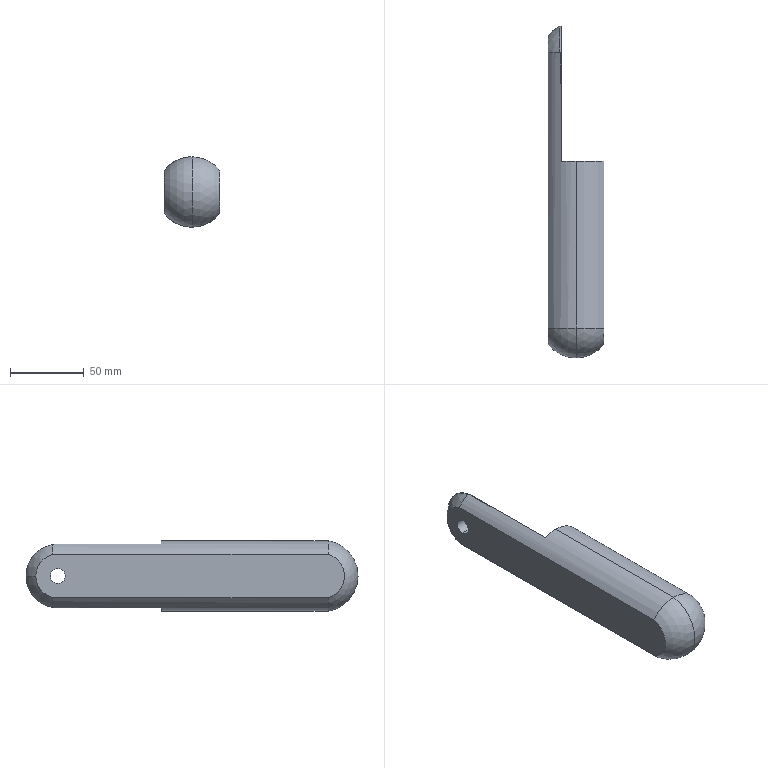Part | SolidWorks | features ICE 12, Fillet 4, RevCut 1, Revolution 1, Scale 1 | 1 solid | 18 faces | box 37.836 x 225.102 x 47.771 mm | volume 229671 mm3 | cylinder 7 | sphere 4 | plane 4 | spline 2 | torus 1 | commonest cylinder face diameters 47.771 x3 1.9 x2 10.1 x2
STEP:
#1=CARTESIAN_POINT('',(18.918,-183.171,14.582));
#2=VERTEX_POINT('',#1);
#3=CARTESIAN_POINT('',(0.,-183.171,23.885));
#4=VERTEX_POINT('',#3);
#5=CARTESIAN_POINT('',(0.,-183.171,0.));
#6=DIRECTION('',(0.,-1.,0.));
#7=DIRECTION('',(0.,0.,-1.));
#8=AXIS2_PLACEMENT_3D('',#5,#6,#7);
#9=CIRCLE('',#8,23.885);
#10=EDGE_CURVE('',#2,#4,#9,.T.);
#11=ORIENTED_EDGE('',*,*,#10,.T.);
#12=CARTESIAN_POINT('',(0.,-203.461,0.));
#13=VERTEX_POINT('',#12);
#14=CARTESIAN_POINT('',(0.,-179.257,0.));
#15=DIRECTION('',(1.,0.,0.));
#16=DIRECTION('',(0.,0.,-1.));
#17=AXIS2_PLACEMENT_3D('',#14,#15,#16);
#18=CIRCLE('',#17,24.204);
#19=EDGE_CURVE('',#4,#13,#18,.T.);
#20=ORIENTED_EDGE('',*,*,#19,.T.);
#21=CARTESIAN_POINT('',(0.,-183.171,-23.885));
#22=VERTEX_POINT('',#21);
#23=CARTESIAN_POINT('',(0.,-179.257,0.));
#24=DIRECTION('',(-1.,0.,0.));
#25=DIRECTION('',(0.,0.,1.));
#26=AXIS2_PLACEMENT_3D('',#23,#24,#25);
#27=CIRCLE('',#26,24.204);
#28=EDGE_CURVE('',#22,#13,#27,.T.);
#29=ORIENTED_EDGE('',*,*,#28,.F.);
#30=CARTESIAN_POINT('',(18.918,-183.171,-14.582));
#31=VERTEX_POINT('',#30);
#32=CARTESIAN_POINT('',(0.,-183.171,0.));
#33=DIRECTION('',(0.,-1.,0.));
#34=DIRECTION('',(0.,0.,-1.));
#35=AXIS2_PLACEMENT_3D('',#32,#33,#34);
#36=CIRCLE('',#35,23.885);
#37=EDGE_CURVE('',#22,#31,#36,.T.);
#38=ORIENTED_EDGE('',*,*,#37,.T.);
#39=CARTESIAN_POINT('',(18.918,-179.257,0.));
#40=DIRECTION('',(1.,0.,0.));
#41=DIRECTION('',(0.,0.,1.));
#42=AXIS2_PLACEMENT_3D('',#39,#40,#41);
#43=CIRCLE('',#42,15.098);
#44=EDGE_CURVE('',#2,#31,#43,.T.);
#45=ORIENTED_EDGE('',*,*,#44,.F.);
#46=EDGE_LOOP('',(#11,#20,#29,#38,#45));
#47=FACE_OUTER_BOUND('',#46,.T.);
#48=CARTESIAN_POINT('',(0.,-179.257,0.));
#49=DIRECTION('',(1.,0.,0.));
#50=DIRECTION('',(0.,0.,-1.));
#51=AXIS2_PLACEMENT_3D('',#48,#49,#50);
#52=SPHERICAL_SURFACE('',#51,24.204);
#53=ADVANCED_FACE('',(#47),#52,.T.);
#54=CARTESIAN_POINT('',(-10.,0.,5.05));
#55=VERTEX_POINT('',#54);
#56=CARTESIAN_POINT('',(-10.,0.,-5.05));
#57=VERTEX_POINT('',#56);
#58=CARTESIAN_POINT('',(-10.,0.,0.));
#59=DIRECTION('',(1.,0.,0.));
#60=DIRECTION('',(0.,0.,1.));
#61=AXIS2_PLACEMENT_3D('',#58,#59,#60);
#62=CIRCLE('',#61,5.05);
#63=EDGE_CURVE('',#55,#57,#62,.T.);
#64=ORIENTED_EDGE('',*,*,#63,.T.);
#65=CARTESIAN_POINT('',(-18.918,0.,-5.05));
#66=VERTEX_POINT('',#65);
#67=CARTESIAN_POINT('',(21.42,0.,-5.05));
#68=DIRECTION('',(-1.,0.,0.));
#69=VECTOR('',#68,1000.);
#70=LINE('',#67,#69);
#71=EDGE_CURVE('',#57,#66,#70,.T.);
#72=ORIENTED_EDGE('',*,*,#71,.T.);
#73=CARTESIAN_POINT('',(-18.918,0.,5.05));
#74=VERTEX_POINT('',#73);
#75=CARTESIAN_POINT('',(-18.918,0.,0.));
#76=DIRECTION('',(-1.,0.,0.));
#77=DIRECTION('',(0.,0.,-1.));
#78=AXIS2_PLACEMENT_3D('',#75,#76,#77);
#79=CIRCLE('',#78,5.05);
#80=EDGE_CURVE('',#66,#74,#79,.T.);
#81=ORIENTED_EDGE('',*,*,#80,.T.);
#82=CARTESIAN_POINT('',(21.42,0.,5.05));
#83=DIRECTION('',(-1.,0.,0.));
#84=VECTOR('',#83,1000.);
#85=LINE('',#82,#84);
#86=EDGE_CURVE('',#55,#74,#85,.T.);
#87=ORIENTED_EDGE('',*,*,#86,.F.);
#88=EDGE_LOOP('',(#64,#72,#81,#87));
#89=FACE_OUTER_BOUND('',#88,.T.);
#90=CARTESIAN_POINT('',(21.42,0.,0.));
#91=DIRECTION('',(-1.,0.,0.));
#92=DIRECTION('',(0.,0.,1.));
#93=AXIS2_PLACEMENT_3D('',#90,#91,#92);
#94=CYLINDRICAL_SURFACE('',#93,5.05);
#95=ADVANCED_FACE('',(#89),#94,.F.);
#96=CARTESIAN_POINT('',(-18.918,3.427,-14.582));
#97=VERTEX_POINT('',#96);
#98=CARTESIAN_POINT('',(-18.918,14.979,0.));
#99=VERTEX_POINT('',#98);
#100=CARTESIAN_POINT('',(-18.918,0.,0.));
#101=DIRECTION('',(1.,0.,0.));
#102=DIRECTION('',(0.,0.,-1.));
#103=AXIS2_PLACEMENT_3D('',#100,#101,#102);
#104=CIRCLE('',#103,14.979);
#105=EDGE_CURVE('',#97,#99,#104,.T.);
#106=ORIENTED_EDGE('',*,*,#105,.T.);
#107=CARTESIAN_POINT('',(-10.878,21.539,0.));
#108=VERTEX_POINT('',#107);
#109=CARTESIAN_POINT('',(0.,0.,0.));
#110=DIRECTION('',(0.,0.,-1.));
#111=DIRECTION('',(-1.,0.,0.));
#112=AXIS2_PLACEMENT_3D('',#109,#110,#111);
#113=CIRCLE('',#112,24.13);
#114=EDGE_CURVE('',#99,#108,#113,.T.);
#115=ORIENTED_EDGE('',*,*,#114,.T.);
#116=CARTESIAN_POINT('',(-10.878,3.427,-21.264));
#117=VERTEX_POINT('',#116);
#118=CARTESIAN_POINT('',(-10.878,0.,0.));
#119=DIRECTION('',(-1.,0.,0.));
#120=DIRECTION('',(0.,1.,0.));
#121=AXIS2_PLACEMENT_3D('',#118,#119,#120);
#122=CIRCLE('',#121,21.539);
#123=EDGE_CURVE('',#108,#117,#122,.T.);
#124=ORIENTED_EDGE('',*,*,#123,.T.);
#125=CARTESIAN_POINT('',(0.,3.427,0.));
#126=DIRECTION('',(0.,1.,0.));
#127=DIRECTION('',(0.,0.,-1.));
#128=AXIS2_PLACEMENT_3D('',#125,#126,#127);
#129=CIRCLE('',#128,23.885);
#130=EDGE_CURVE('',#117,#97,#129,.T.);
#131=ORIENTED_EDGE('',*,*,#130,.T.);
#132=EDGE_LOOP('',(#106,#115,#124,#131));
#133=FACE_OUTER_BOUND('',#132,.T.);
#134=CARTESIAN_POINT('',(0.,0.,0.));
#135=DIRECTION('',(0.,0.,-1.));
#136=DIRECTION('',(1.,0.,0.));
#137=AXIS2_PLACEMENT_3D('',#134,#135,#136);
#138=SPHERICAL_SURFACE('',#137,24.13);
#139=ADVANCED_FACE('',(#133),#138,.T.);
#140=CARTESIAN_POINT('',(-18.918,-183.171,14.582));
#141=VERTEX_POINT('',#140);
#142=CARTESIAN_POINT('',(0.,-183.171,0.));
#143=DIRECTION('',(0.,-1.,0.));
#144=DIRECTION('',(0.,0.,-1.));
#145=AXIS2_PLACEMENT_3D('',#142,#143,#144);
#146=CIRCLE('',#145,23.885);
#147=EDGE_CURVE('',#4,#141,#146,.T.);
#148=ORIENTED_EDGE('',*,*,#147,.F.);
#149=CARTESIAN_POINT('',(0.,-70.,23.885));
#150=VERTEX_POINT('',#149);
#151=CARTESIAN_POINT('',(0.,-127.87,23.885));
#152=DIRECTION('',(0.,1.,0.));
#153=VECTOR('',#152,1000.);
#154=LINE('',#151,#153);
#155=EDGE_CURVE('',#4,#150,#154,.T.);
#156=ORIENTED_EDGE('',*,*,#155,.T.);
#157=CARTESIAN_POINT('',(-10.,-70.,21.691));
#158=VERTEX_POINT('',#157);
#159=CARTESIAN_POINT('',(0.,-70.,0.));
#160=DIRECTION('',(0.,1.,0.));
#161=DIRECTION('',(0.,0.,-1.));
#162=AXIS2_PLACEMENT_3D('',#159,#160,#161);
#163=CIRCLE('',#162,23.885);
#164=EDGE_CURVE('',#158,#150,#163,.T.);
#165=ORIENTED_EDGE('',*,*,#164,.F.);
#166=CARTESIAN_POINT('',(-10.,-18.195,21.691));
#167=VERTEX_POINT('',#166);
#168=CARTESIAN_POINT('',(-10.,-127.87,21.691));
#169=DIRECTION('',(0.,-1.,0.));
#170=VECTOR('',#169,1000.);
#171=LINE('',#168,#170);
#172=EDGE_CURVE('',#167,#158,#171,.T.);
#173=ORIENTED_EDGE('',*,*,#172,.F.);
#174=CARTESIAN_POINT('',(-10.187,-17.296,21.604));
#175=VERTEX_POINT('',#174);
#176=CARTESIAN_POINT('',(-10.187,-17.296,21.604));
#177=CARTESIAN_POINT('',(-10.187,-17.452,21.604));
#178=CARTESIAN_POINT('',(-10.175,-17.607,21.61));
#179=CARTESIAN_POINT('',(-10.118,-17.909,21.636));
#180=CARTESIAN_POINT('',(-10.072,-18.06,21.658));
#181=CARTESIAN_POINT('',(-10.,-18.195,21.691));
#182=B_SPLINE_CURVE_WITH_KNOTS('',3,(#176,#177,#178,#179,#180,#181),.UNSPECIFIED.,.F.,.F.,(4,2,4),(0.,0.0004629,0.0009257),.UNSPECIFIED.);
#183=EDGE_CURVE('',#175,#167,#182,.T.);
#184=ORIENTED_EDGE('',*,*,#183,.F.);
#185=CARTESIAN_POINT('',(-10.187,0.,21.604));
#186=VERTEX_POINT('',#185);
#187=CARTESIAN_POINT('',(-10.187,-53.115,21.604));
#188=DIRECTION('',(0.,-1.,0.));
#189=VECTOR('',#188,1000.);
#190=LINE('',#187,#189);
#191=EDGE_CURVE('',#186,#175,#190,.T.);
#192=ORIENTED_EDGE('',*,*,#191,.F.);
#193=CARTESIAN_POINT('',(-10.878,3.427,21.264));
#194=VERTEX_POINT('',#193);
#195=CARTESIAN_POINT('',(-10.878,3.427,21.264));
#196=CARTESIAN_POINT('',(-10.844,3.427,21.282));
#197=CARTESIAN_POINT('',(-10.811,3.411,21.299));
#198=CARTESIAN_POINT('',(-10.755,3.366,21.327));
#199=CARTESIAN_POINT('',(-10.731,3.339,21.339));
#200=CARTESIAN_POINT('',(-10.667,3.249,21.371));
#201=CARTESIAN_POINT('',(-10.633,3.182,21.388));
#202=CARTESIAN_POINT('',(-10.543,2.979,21.433));
#203=CARTESIAN_POINT('',(-10.498,2.834,21.455));
#204=CARTESIAN_POINT('',(-10.384,2.398,21.51));
#205=CARTESIAN_POINT('',(-10.334,2.102,21.534));
#206=CARTESIAN_POINT('',(-10.218,1.21,21.59));
#207=CARTESIAN_POINT('',(-10.187,0.6043,21.604));
#208=CARTESIAN_POINT('',(-10.187,0.,21.604));
#209=B_SPLINE_CURVE_WITH_KNOTS('',3,(#195,#196,#197,#198,#199,#200,#201,#202,#203,#204,#205,#206,#207,#208),.UNSPECIFIED.,.F.,.F.,(4,2,2,2,2,2,4),(0.000000221,0.0001151,0.00023,0.0004598,0.0009194,0.001839,0.003677),.UNSPECIFIED.);
#210=EDGE_CURVE('',#194,#186,#209,.T.);
#211=ORIENTED_EDGE('',*,*,#210,.F.);
#212=CARTESIAN_POINT('',(-18.918,3.427,14.582));
#213=VERTEX_POINT('',#212);
#214=CARTESIAN_POINT('',(0.,3.427,0.));
#215=DIRECTION('',(0.,1.,0.));
#216=DIRECTION('',(0.,0.,-1.));
#217=AXIS2_PLACEMENT_3D('',#214,#215,#216);
#218=CIRCLE('',#217,23.885);
#219=EDGE_CURVE('',#213,#194,#218,.T.);
#220=ORIENTED_EDGE('',*,*,#219,.F.);
#221=CARTESIAN_POINT('',(-18.918,-127.87,14.582));
#222=DIRECTION('',(0.,1.,0.));
#223=VECTOR('',#222,1000.);
#224=LINE('',#221,#223);
#225=EDGE_CURVE('',#141,#213,#224,.T.);
#226=ORIENTED_EDGE('',*,*,#225,.F.);
#227=EDGE_LOOP('',(#148,#156,#165,#173,#184,#192,#211,#220,#226));
#228=FACE_OUTER_BOUND('',#227,.T.);
#229=CARTESIAN_POINT('',(0.,-127.87,0.));
#230=DIRECTION('',(0.,1.,0.));
#231=DIRECTION('',(0.,0.,1.));
#232=AXIS2_PLACEMENT_3D('',#229,#230,#231);
#233=CYLINDRICAL_SURFACE('',#232,23.885);
#234=ADVANCED_FACE('',(#228),#233,.T.);
#235=CARTESIAN_POINT('',(-18.918,-183.171,-14.582));
#236=VERTEX_POINT('',#235);
#237=CARTESIAN_POINT('',(-18.918,-127.87,-14.582));
#238=DIRECTION('',(0.,-1.,0.));
#239=VECTOR('',#238,1000.);
#240=LINE('',#237,#239);
#241=EDGE_CURVE('',#97,#236,#240,.T.);
#242=ORIENTED_EDGE('',*,*,#241,.F.);
#243=ORIENTED_EDGE('',*,*,#130,.F.);
#244=CARTESIAN_POINT('',(-10.187,0.,-21.604));
#245=VERTEX_POINT('',#244);
#246=CARTESIAN_POINT('',(-10.187,0.,-21.604));
#247=CARTESIAN_POINT('',(-10.187,0.6048,-21.604));
#248=CARTESIAN_POINT('',(-10.217,1.207,-21.59));
#249=CARTESIAN_POINT('',(-10.334,2.105,-21.534));
#250=CARTESIAN_POINT('',(-10.385,2.404,-21.51));
#251=CARTESIAN_POINT('',(-10.5,2.839,-21.454));
#252=CARTESIAN_POINT('',(-10.545,2.983,-21.432));
#253=CARTESIAN_POINT('',(-10.635,3.186,-21.387));
#254=CARTESIAN_POINT('',(-10.669,3.252,-21.37));
#255=CARTESIAN_POINT('',(-10.733,3.34,-21.338));
#256=CARTESIAN_POINT('',(-10.756,3.368,-21.326));
#257=CARTESIAN_POINT('',(-10.812,3.411,-21.298));
#258=CARTESIAN_POINT('',(-10.844,3.427,-21.282));
#259=CARTESIAN_POINT('',(-10.878,3.427,-21.264));
#260=B_SPLINE_CURVE_WITH_KNOTS('',3,(#246,#247,#248,#249,#250,#251,#252,#253,#254,#255,#256,#257,#258,#259),.UNSPECIFIED.,.F.,.F.,(4,2,2,2,2,2,4),(0.0000002,0.00181,0.002715,0.003167,0.003394,0.003507,0.00362),.UNSPECIFIED.);
#261=EDGE_CURVE('',#245,#117,#260,.T.);
#262=ORIENTED_EDGE('',*,*,#261,.F.);
#263=CARTESIAN_POINT('',(-10.187,-58.677,-21.604));
#264=VERTEX_POINT('',#263);
#265=CARTESIAN_POINT('',(-10.187,-53.115,-21.604));
#266=DIRECTION('',(0.,1.,0.));
#267=VECTOR('',#266,1000.);
#268=LINE('',#265,#267);
#269=EDGE_CURVE('',#264,#245,#268,.T.);
#270=ORIENTED_EDGE('',*,*,#269,.F.);
#271=CARTESIAN_POINT('',(-10.,-59.803,-21.691));
#272=VERTEX_POINT('',#271);
#273=CARTESIAN_POINT('',(-10.,-59.803,-21.691));
#274=CARTESIAN_POINT('',(-10.058,-59.623,-21.664));
#275=CARTESIAN_POINT('',(-10.105,-59.436,-21.643));
#276=CARTESIAN_POINT('',(-10.169,-59.061,-21.613));
#277=CARTESIAN_POINT('',(-10.187,-58.871,-21.604));
#278=CARTESIAN_POINT('',(-10.187,-58.677,-21.604));
#279=B_SPLINE_CURVE_WITH_KNOTS('',3,(#273,#274,#275,#276,#277,#278),.UNSPECIFIED.,.F.,.F.,(4,2,4),(0.00244,0.003016,0.003592),.UNSPECIFIED.);
#280=EDGE_CURVE('',#272,#264,#279,.T.);
#281=ORIENTED_EDGE('',*,*,#280,.F.);
#282=CARTESIAN_POINT('',(-10.,-70.,-21.691));
#283=VERTEX_POINT('',#282);
#284=CARTESIAN_POINT('',(-10.,-127.87,-21.691));
#285=DIRECTION('',(0.,1.,0.));
#286=VECTOR('',#285,1000.);
#287=LINE('',#284,#286);
#288=EDGE_CURVE('',#283,#272,#287,.T.);
#289=ORIENTED_EDGE('',*,*,#288,.F.);
#290=CARTESIAN_POINT('',(18.918,-70.,-14.582));
#291=VERTEX_POINT('',#290);
#292=CARTESIAN_POINT('',(0.,-70.,0.));
#293=DIRECTION('',(0.,1.,0.));
#294=DIRECTION('',(0.,0.,-1.));
#295=AXIS2_PLACEMENT_3D('',#292,#293,#294);
#296=CIRCLE('',#295,23.885);
#297=EDGE_CURVE('',#291,#283,#296,.T.);
#298=ORIENTED_EDGE('',*,*,#297,.F.);
#299=CARTESIAN_POINT('',(18.918,-127.87,-14.582));
#300=DIRECTION('',(0.,1.,0.));
#301=VECTOR('',#300,1000.);
#302=LINE('',#299,#301);
#303=EDGE_CURVE('',#31,#291,#302,.T.);
#304=ORIENTED_EDGE('',*,*,#303,.F.);
#305=ORIENTED_EDGE('',*,*,#37,.F.);
#306=CARTESIAN_POINT('',(0.,-183.171,0.));
#307=DIRECTION('',(0.,-1.,0.));
#308=DIRECTION('',(0.,0.,-1.));
#309=AXIS2_PLACEMENT_3D('',#306,#307,#308);
#310=CIRCLE('',#309,23.885);
#311=EDGE_CURVE('',#236,#22,#310,.T.);
#312=ORIENTED_EDGE('',*,*,#311,.F.);
#313=EDGE_LOOP('',(#242,#243,#262,#270,#281,#289,#298,#304,#305,#312));
#314=FACE_OUTER_BOUND('',#313,.T.);
#315=CARTESIAN_POINT('',(0.,-127.87,0.));
#316=DIRECTION('',(0.,1.,0.));
#317=DIRECTION('',(0.,0.,1.));
#318=AXIS2_PLACEMENT_3D('',#315,#316,#317);
#319=CYLINDRICAL_SURFACE('',#318,23.885);
#320=ADVANCED_FACE('',(#314),#319,.T.);
#321=ORIENTED_EDGE('',*,*,#155,.F.);
#322=ORIENTED_EDGE('',*,*,#10,.F.);
#323=CARTESIAN_POINT('',(18.918,-70.,14.582));
#324=VERTEX_POINT('',#323);
#325=CARTESIAN_POINT('',(18.918,-127.87,14.582));
#326=DIRECTION('',(0.,-1.,0.));
#327=VECTOR('',#326,1000.);
#328=LINE('',#325,#327);
#329=EDGE_CURVE('',#324,#2,#328,.T.);
#330=ORIENTED_EDGE('',*,*,#329,.F.);
#331=CARTESIAN_POINT('',(0.,-70.,0.));
#332=DIRECTION('',(0.,1.,0.));
#333=DIRECTION('',(0.,0.,-1.));
#334=AXIS2_PLACEMENT_3D('',#331,#332,#333);
#335=CIRCLE('',#334,23.885);
#336=EDGE_CURVE('',#150,#324,#335,.T.);
#337=ORIENTED_EDGE('',*,*,#336,.F.);
#338=EDGE_LOOP('',(#321,#322,#330,#337));
#339=FACE_OUTER_BOUND('',#338,.T.);
#340=CARTESIAN_POINT('',(0.,-127.87,0.));
#341=DIRECTION('',(0.,1.,0.));
#342=DIRECTION('',(0.,0.,1.));
#343=AXIS2_PLACEMENT_3D('',#340,#341,#342);
#344=CYLINDRICAL_SURFACE('',#343,23.885);
#345=ADVANCED_FACE('',(#339),#344,.T.);
#346=ORIENTED_EDGE('',*,*,#114,.F.);
#347=CARTESIAN_POINT('',(-18.918,0.,0.));
#348=DIRECTION('',(1.,0.,0.));
#349=DIRECTION('',(0.,0.,-1.));
#350=AXIS2_PLACEMENT_3D('',#347,#348,#349);
#351=CIRCLE('',#350,14.979);
#352=EDGE_CURVE('',#99,#213,#351,.T.);
#353=ORIENTED_EDGE('',*,*,#352,.T.);
#354=ORIENTED_EDGE('',*,*,#219,.T.);
#355=CARTESIAN_POINT('',(-10.878,0.,0.));
#356=DIRECTION('',(-1.,0.,0.));
#357=DIRECTION('',(0.,1.,0.));
#358=AXIS2_PLACEMENT_3D('',#355,#356,#357);
#359=CIRCLE('',#358,21.539);
#360=EDGE_CURVE('',#194,#108,#359,.T.);
#361=ORIENTED_EDGE('',*,*,#360,.T.);
#362=EDGE_LOOP('',(#346,#353,#354,#361));
#363=FACE_OUTER_BOUND('',#362,.T.);
#364=CARTESIAN_POINT('',(0.,0.,0.));
#365=DIRECTION('',(0.,0.,-1.));
#366=DIRECTION('',(1.,0.,0.));
#367=AXIS2_PLACEMENT_3D('',#364,#365,#366);
#368=SPHERICAL_SURFACE('',#367,24.13);
#369=ADVANCED_FACE('',(#363),#368,.T.);
#370=CARTESIAN_POINT('',(-10.,0.,21.527));
#371=VERTEX_POINT('',#370);
#372=CARTESIAN_POINT('',(-10.,-17.296,21.527));
#373=VERTEX_POINT('',#372);
#374=CARTESIAN_POINT('',(-10.,24.13,21.527));
#375=DIRECTION('',(0.,-1.,0.));
#376=VECTOR('',#375,1000.);
#377=LINE('',#374,#376);
#378=EDGE_CURVE('',#371,#373,#377,.T.);
#379=ORIENTED_EDGE('',*,*,#378,.F.);
#380=CARTESIAN_POINT('',(-10.45,0.,20.691));
#381=DIRECTION('',(0.,1.,0.));
#382=DIRECTION('',(-1.,0.,0.));
#383=AXIS2_PLACEMENT_3D('',#380,#381,#382);
#384=CIRCLE('',#383,0.95);
#385=EDGE_CURVE('',#186,#371,#384,.T.);
#386=ORIENTED_EDGE('',*,*,#385,.F.);
#387=ORIENTED_EDGE('',*,*,#191,.T.);
#388=CARTESIAN_POINT('',(-10.45,-17.296,20.691));
#389=DIRECTION('',(0.,-1.,0.));
#390=DIRECTION('',(0.,0.,-1.));
#391=AXIS2_PLACEMENT_3D('',#388,#389,#390);
#392=CIRCLE('',#391,0.95);
#393=EDGE_CURVE('',#373,#175,#392,.T.);
#394=ORIENTED_EDGE('',*,*,#393,.F.);
#395=EDGE_LOOP('',(#379,#386,#387,#394));
#396=FACE_OUTER_BOUND('',#395,.T.);
#397=CARTESIAN_POINT('',(-10.45,24.13,20.691));
#398=DIRECTION('',(0.,1.,0.));
#399=DIRECTION('',(-1.,0.,0.));
#400=AXIS2_PLACEMENT_3D('',#397,#398,#399);
#401=CYLINDRICAL_SURFACE('',#400,0.95);
#402=ADVANCED_FACE('',(#396),#401,.T.);
#403=CARTESIAN_POINT('',(-10.,-17.296,21.527));
#404=CARTESIAN_POINT('',(-10.,-17.45,21.527));
#405=CARTESIAN_POINT('',(-10.,-17.603,21.54));
#406=CARTESIAN_POINT('',(-10.,-17.902,21.596));
#407=CARTESIAN_POINT('',(-10.,-18.05,21.638));
#408=CARTESIAN_POINT('',(-10.,-18.195,21.691));
#409=B_SPLINE_CURVE_WITH_KNOTS('',3,(#403,#404,#405,#406,#407,#408),.UNSPECIFIED.,.F.,.F.,(4,2,4),(0.,0.0004571,0.0009143),.UNSPECIFIED.);
#410=EDGE_CURVE('',#373,#167,#409,.T.);
#411=ORIENTED_EDGE('',*,*,#410,.F.);
#412=ORIENTED_EDGE('',*,*,#393,.T.);
#413=ORIENTED_EDGE('',*,*,#183,.T.);
#414=EDGE_LOOP('',(#411,#412,#413));
#415=FACE_OUTER_BOUND('',#414,.T.);
#416=CARTESIAN_POINT('',(-10.277,-17.296,21.625));
#417=CARTESIAN_POINT('',(-10.13,-17.296,21.598));
#418=CARTESIAN_POINT('',(-9.998,-17.296,21.526));
#419=CARTESIAN_POINT('',(-10.262,-17.475,21.622));
#420=CARTESIAN_POINT('',(-10.11,-17.467,21.591));
#421=CARTESIAN_POINT('',(-9.976,-17.462,21.514));
#422=CARTESIAN_POINT('',(-10.231,-17.643,21.627));
#423=CARTESIAN_POINT('',(-10.076,-17.627,21.592));
#424=CARTESIAN_POINT('',(-9.939,-17.616,21.509));
#425=CARTESIAN_POINT('',(-10.139,-17.952,21.65));
#426=CARTESIAN_POINT('',(-9.98,-17.914,21.606));
#427=CARTESIAN_POINT('',(-9.843,-17.889,21.509));
#428=CARTESIAN_POINT('',(-10.077,-18.092,21.67));
#429=CARTESIAN_POINT('',(-9.917,-18.041,21.62));
#430=CARTESIAN_POINT('',(-9.781,-18.009,21.515));
#431=CARTESIAN_POINT('',(-10.004,-18.202,21.695));
#432=CARTESIAN_POINT('',(-9.849,-18.136,21.638));
#433=CARTESIAN_POINT('',(-9.717,-18.097,21.525));
#434=(BOUNDED_SURFACE()B_SPLINE_SURFACE(3,2,((#416,#417,#418),(#419,#420,#421),(#422,#423,#424),(#425,#426,#427),(#428,#429,#430),(#431,#432,#433)),.UNSPECIFIED.,.F.,.F.,.T.)B_SPLINE_SURFACE_WITH_KNOTS((4,2,4),(3,3),(-0.002813,-0.002178,-0.001543),(0.3332,0.4753),.UNSPECIFIED.)GEOMETRIC_REPRESENTATION_ITEM()RATIONAL_B_SPLINE_SURFACE(((0.7885,0.7659,0.7626),(0.7779,0.7542,0.7507),(0.7672,0.7424,0.7387),(0.7465,0.7195,0.7154),(0.7363,0.7082,0.704),(0.7279,0.6988,0.6945)))REPRESENTATION_ITEM('')SURFACE());
#435=ADVANCED_FACE('',(#415),#434,.T.);
#436=CARTESIAN_POINT('',(-10.,0.,-21.527));
#437=VERTEX_POINT('',#436);
#438=CARTESIAN_POINT('',(-10.,0.,0.));
#439=DIRECTION('',(1.,0.,0.));
#440=DIRECTION('',(0.,0.,1.));
#441=AXIS2_PLACEMENT_3D('',#438,#439,#440);
#442=CIRCLE('',#441,21.527);
#443=EDGE_CURVE('',#437,#371,#442,.T.);
#444=ORIENTED_EDGE('',*,*,#443,.F.);
#445=CARTESIAN_POINT('',(-10.45,0.,-20.691));
#446=DIRECTION('',(0.,-1.,0.));
#447=DIRECTION('',(0.,0.,-1.));
#448=AXIS2_PLACEMENT_3D('',#445,#446,#447);
#449=CIRCLE('',#448,0.95);
#450=EDGE_CURVE('',#245,#437,#449,.T.);
#451=ORIENTED_EDGE('',*,*,#450,.F.);
#452=ORIENTED_EDGE('',*,*,#261,.T.);
#453=ORIENTED_EDGE('',*,*,#123,.F.);
#454=ORIENTED_EDGE('',*,*,#360,.F.);
#455=ORIENTED_EDGE('',*,*,#210,.T.);
#456=ORIENTED_EDGE('',*,*,#385,.T.);
#457=EDGE_LOOP('',(#444,#451,#452,#453,#454,#455,#456));
#458=FACE_OUTER_BOUND('',#457,.T.);
#459=CARTESIAN_POINT('',(-10.45,0.,0.));
#460=DIRECTION('',(-1.,0.,0.));
#461=DIRECTION('',(0.,-1.,0.));
#462=AXIS2_PLACEMENT_3D('',#459,#460,#461);
#463=TOROIDAL_SURFACE('',#462,20.691,0.95);
#464=ADVANCED_FACE('',(#458),#463,.T.);
#465=CARTESIAN_POINT('',(-10.,-58.677,-21.527));
#466=VERTEX_POINT('',#465);
#467=CARTESIAN_POINT('',(-10.,24.13,-21.527));
#468=DIRECTION('',(0.,1.,0.));
#469=VECTOR('',#468,1000.);
#470=LINE('',#467,#469);
#471=EDGE_CURVE('',#466,#437,#470,.T.);
#472=ORIENTED_EDGE('',*,*,#471,.F.);
#473=CARTESIAN_POINT('',(-10.45,-58.677,-20.691));
#474=DIRECTION('',(0.,-1.,0.));
#475=DIRECTION('',(0.,0.,-1.));
#476=AXIS2_PLACEMENT_3D('',#473,#474,#475);
#477=CIRCLE('',#476,0.95);
#478=EDGE_CURVE('',#264,#466,#477,.T.);
#479=ORIENTED_EDGE('',*,*,#478,.F.);
#480=ORIENTED_EDGE('',*,*,#269,.T.);
#481=ORIENTED_EDGE('',*,*,#450,.T.);
#482=EDGE_LOOP('',(#472,#479,#480,#481));
#483=FACE_OUTER_BOUND('',#482,.T.);
#484=CARTESIAN_POINT('',(-10.45,24.13,-20.691));
#485=DIRECTION('',(0.,1.,0.));
#486=DIRECTION('',(-1.,0.,0.));
#487=AXIS2_PLACEMENT_3D('',#484,#485,#486);
#488=CYLINDRICAL_SURFACE('',#487,0.95);
#489=ADVANCED_FACE('',(#483),#488,.T.);
#490=CARTESIAN_POINT('',(-10.,-59.803,-21.691));
#491=CARTESIAN_POINT('',(-10.,-59.434,-21.604));
#492=CARTESIAN_POINT('',(-10.,-59.062,-21.527));
#493=CARTESIAN_POINT('',(-10.,-58.677,-21.527));
#494=B_SPLINE_CURVE_WITH_KNOTS('',3,(#490,#491,#492,#493),.UNSPECIFIED.,.F.,.F.,(4,4),(0.001535,0.002671),.UNSPECIFIED.);
#495=EDGE_CURVE('',#272,#466,#494,.T.);
#496=ORIENTED_EDGE('',*,*,#495,.F.);
#497=ORIENTED_EDGE('',*,*,#280,.T.);
#498=ORIENTED_EDGE('',*,*,#478,.T.);
#499=EDGE_LOOP('',(#496,#497,#498));
#500=FACE_OUTER_BOUND('',#499,.T.);
#501=CARTESIAN_POINT('',(-9.961,-58.677,-21.505));
#502=CARTESIAN_POINT('',(-10.07,-58.677,-21.571));
#503=CARTESIAN_POINT('',(-10.193,-58.677,-21.605));
#504=CARTESIAN_POINT('',(-9.985,-58.851,-21.52));
#505=CARTESIAN_POINT('',(-10.092,-58.855,-21.58));
#506=CARTESIAN_POINT('',(-10.211,-58.862,-21.61));
#507=CARTESIAN_POINT('',(-9.994,-59.034,-21.541));
#508=CARTESIAN_POINT('',(-10.098,-59.043,-21.596));
#509=CARTESIAN_POINT('',(-10.213,-59.054,-21.623));
#510=CARTESIAN_POINT('',(-9.982,-59.408,-21.595));
#511=CARTESIAN_POINT('',(-10.08,-59.424,-21.641));
#512=CARTESIAN_POINT('',(-10.186,-59.444,-21.663));
#513=CARTESIAN_POINT('',(-9.962,-59.598,-21.627));
#514=CARTESIAN_POINT('',(-10.057,-59.618,-21.669));
#515=CARTESIAN_POINT('',(-10.158,-59.642,-21.689));
#516=CARTESIAN_POINT('',(-9.928,-59.792,-21.666));
#517=CARTESIAN_POINT('',(-10.019,-59.815,-21.704));
#518=CARTESIAN_POINT('',(-10.115,-59.842,-21.722));
#519=(BOUNDED_SURFACE()B_SPLINE_SURFACE(3,2,((#501,#502,#503),(#504,#505,#506),(#507,#508,#509),(#510,#511,#512),(#513,#514,#515),(#516,#517,#518)),.UNSPECIFIED.,.F.,.F.,.F.)B_SPLINE_SURFACE_WITH_KNOTS((4,2,4),(3,3),(0.0009633,0.001646,0.002329),(0.5048,0.6248),.UNSPECIFIED.)GEOMETRIC_REPRESENTATION_ITEM()RATIONAL_B_SPLINE_SURFACE(((0.762,0.7626,0.7768),(0.775,0.7755,0.789),(0.7875,0.788,0.8007),(0.812,0.8124,0.8237),(0.8238,0.8243,0.8348),(0.8355,0.8358,0.8457)))REPRESENTATION_ITEM('')SURFACE());
#520=ADVANCED_FACE('',(#500),#519,.T.);
#521=ORIENTED_EDGE('',*,*,#71,.F.);
#522=CARTESIAN_POINT('',(-10.,0.,0.));
#523=DIRECTION('',(1.,0.,0.));
#524=DIRECTION('',(0.,0.,1.));
#525=AXIS2_PLACEMENT_3D('',#522,#523,#524);
#526=CIRCLE('',#525,5.05);
#527=EDGE_CURVE('',#57,#55,#526,.T.);
#528=ORIENTED_EDGE('',*,*,#527,.T.);
#529=ORIENTED_EDGE('',*,*,#86,.T.);
#530=CARTESIAN_POINT('',(-18.918,0.,0.));
#531=DIRECTION('',(-1.,0.,0.));
#532=DIRECTION('',(0.,0.,-1.));
#533=AXIS2_PLACEMENT_3D('',#530,#531,#532);
#534=CIRCLE('',#533,5.05);
#535=EDGE_CURVE('',#74,#66,#534,.T.);
#536=ORIENTED_EDGE('',*,*,#535,.T.);
#537=EDGE_LOOP('',(#521,#528,#529,#536));
#538=FACE_OUTER_BOUND('',#537,.T.);
#539=CARTESIAN_POINT('',(21.42,0.,0.));
#540=DIRECTION('',(-1.,0.,0.));
#541=DIRECTION('',(0.,0.,1.));
#542=AXIS2_PLACEMENT_3D('',#539,#540,#541);
#543=CYLINDRICAL_SURFACE('',#542,5.05);
#544=ADVANCED_FACE('',(#538),#543,.F.);
#545=ORIENTED_EDGE('',*,*,#19,.F.);
#546=ORIENTED_EDGE('',*,*,#147,.T.);
#547=CARTESIAN_POINT('',(-18.918,-179.257,0.));
#548=DIRECTION('',(-1.,0.,0.));
#549=DIRECTION('',(0.,0.,-1.));
#550=AXIS2_PLACEMENT_3D('',#547,#548,#549);
#551=CIRCLE('',#550,15.098);
#552=EDGE_CURVE('',#236,#141,#551,.T.);
#553=ORIENTED_EDGE('',*,*,#552,.F.);
#554=ORIENTED_EDGE('',*,*,#311,.T.);
#555=ORIENTED_EDGE('',*,*,#28,.T.);
#556=EDGE_LOOP('',(#545,#546,#553,#554,#555));
#557=FACE_OUTER_BOUND('',#556,.T.);
#558=CARTESIAN_POINT('',(0.,-179.257,0.));
#559=DIRECTION('',(1.,0.,0.));
#560=DIRECTION('',(0.,0.,-1.));
#561=AXIS2_PLACEMENT_3D('',#558,#559,#560);
#562=SPHERICAL_SURFACE('',#561,24.204);
#563=ADVANCED_FACE('',(#557),#562,.T.);
#564=ORIENTED_EDGE('',*,*,#172,.T.);
#565=CARTESIAN_POINT('',(-10.,-70.,-23.885));
#566=DIRECTION('',(0.,0.,1.));
#567=VECTOR('',#566,1000.);
#568=LINE('',#565,#567);
#569=EDGE_CURVE('',#283,#158,#568,.T.);
#570=ORIENTED_EDGE('',*,*,#569,.F.);
#571=ORIENTED_EDGE('',*,*,#288,.T.);
#572=ORIENTED_EDGE('',*,*,#495,.T.);
#573=ORIENTED_EDGE('',*,*,#471,.T.);
#574=ORIENTED_EDGE('',*,*,#443,.T.);
#575=ORIENTED_EDGE('',*,*,#378,.T.);
#576=ORIENTED_EDGE('',*,*,#410,.T.);
#577=EDGE_LOOP('',(#564,#570,#571,#572,#573,#574,#575,#576));
#578=FACE_OUTER_BOUND('',#577,.T.);
#579=ORIENTED_EDGE('',*,*,#63,.F.);
#580=ORIENTED_EDGE('',*,*,#527,.F.);
#581=EDGE_LOOP('',(#579,#580));
#582=FACE_BOUND('',#581,.T.);
#583=CARTESIAN_POINT('',(-10.,-70.,-23.885));
#584=DIRECTION('',(-1.,0.,0.));
#585=DIRECTION('',(0.,0.,1.));
#586=AXIS2_PLACEMENT_3D('',#583,#584,#585);
#587=PLANE('',#586);
#588=ADVANCED_FACE('',(#578,#582),#587,.F.);
#589=ORIENTED_EDGE('',*,*,#164,.T.);
#590=ORIENTED_EDGE('',*,*,#336,.T.);
#591=CARTESIAN_POINT('',(18.918,-70.,-23.885));
#592=DIRECTION('',(0.,0.,-1.));
#593=VECTOR('',#592,1000.);
#594=LINE('',#591,#593);
#595=EDGE_CURVE('',#324,#291,#594,.T.);
#596=ORIENTED_EDGE('',*,*,#595,.T.);
#597=ORIENTED_EDGE('',*,*,#297,.T.);
#598=ORIENTED_EDGE('',*,*,#569,.T.);
#599=EDGE_LOOP('',(#589,#590,#596,#597,#598));
#600=FACE_OUTER_BOUND('',#599,.T.);
#601=CARTESIAN_POINT('',(-10.,-70.,-23.885));
#602=DIRECTION('',(0.,-1.,0.));
#603=DIRECTION('',(0.,0.,-1.));
#604=AXIS2_PLACEMENT_3D('',#601,#602,#603);
#605=PLANE('',#604);
#606=ADVANCED_FACE('',(#600),#605,.F.);
#607=ORIENTED_EDGE('',*,*,#44,.T.);
#608=ORIENTED_EDGE('',*,*,#303,.T.);
#609=ORIENTED_EDGE('',*,*,#595,.F.);
#610=ORIENTED_EDGE('',*,*,#329,.T.);
#611=EDGE_LOOP('',(#607,#608,#609,#610));
#612=FACE_OUTER_BOUND('',#611,.T.);
#613=CARTESIAN_POINT('',(18.918,-231.652,-23.885));
#614=DIRECTION('',(-1.,0.,0.));
#615=DIRECTION('',(0.,0.,1.));
#616=AXIS2_PLACEMENT_3D('',#613,#614,#615);
#617=PLANE('',#616);
#618=ADVANCED_FACE('',(#612),#617,.F.);
#619=ORIENTED_EDGE('',*,*,#105,.F.);
#620=ORIENTED_EDGE('',*,*,#241,.T.);
#621=ORIENTED_EDGE('',*,*,#552,.T.);
#622=ORIENTED_EDGE('',*,*,#225,.T.);
#623=ORIENTED_EDGE('',*,*,#352,.F.);
#624=EDGE_LOOP('',(#619,#620,#621,#622,#623));
#625=FACE_OUTER_BOUND('',#624,.T.);
#626=ORIENTED_EDGE('',*,*,#535,.F.);
#627=ORIENTED_EDGE('',*,*,#80,.F.);
#628=EDGE_LOOP('',(#626,#627));
#629=FACE_BOUND('',#628,.T.);
#630=CARTESIAN_POINT('',(-18.918,-231.652,-23.885));
#631=DIRECTION('',(1.,0.,0.));
#632=DIRECTION('',(0.,0.,-1.));
#633=AXIS2_PLACEMENT_3D('',#630,#631,#632);
#634=PLANE('',#633);
#635=ADVANCED_FACE('',(#625,#629),#634,.F.);
#636=CLOSED_SHELL('',(#53,#95,#139,#234,#320,#345,#369,#402,#435,#464,#489,#520,#544,#563,#588,#606,#618,#635));
#637=MANIFOLD_SOLID_BREP('',#636);
#638=CARTESIAN_POINT('',(0.,0.,0.));
#639=DIRECTION('',(0.,0.,1.));
#640=DIRECTION('',(1.,0.,0.));
#641=AXIS2_PLACEMENT_3D('',#638,#639,#640);
#642=(LENGTH_UNIT()NAMED_UNIT(*)SI_UNIT(.MILLI.,.METRE.));
#643=UNCERTAINTY_MEASURE_WITH_UNIT(LENGTH_MEASURE(0.00001),#642,'','');
#644=(NAMED_UNIT(*)PLANE_ANGLE_UNIT()SI_UNIT($,.RADIAN.));
#645=(NAMED_UNIT(*)SI_UNIT($,.STERADIAN.)SOLID_ANGLE_UNIT());
#646=(GEOMETRIC_REPRESENTATION_CONTEXT(3)GLOBAL_UNCERTAINTY_ASSIGNED_CONTEXT((#643))GLOBAL_UNIT_ASSIGNED_CONTEXT((#642,#644,#645))REPRESENTATION_CONTEXT('',''));
#647=ADVANCED_BREP_SHAPE_REPRESENTATION('',(#637,#641),#646);